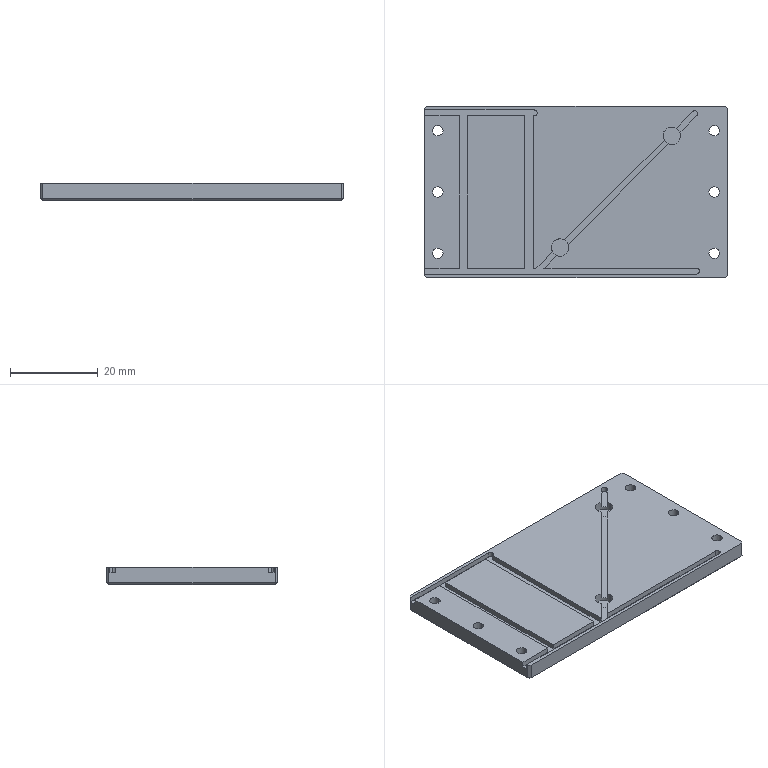Part | STEP file | ASND-0110-OPT-CO40-X-V1.0.5 side plate | 1 solid | 78 faces | box 69 x 39 x 4 mm | volume 10181 mm3 | plane 44 | cylinder 22 | cone 12 | commonest cylinder face diameters 2.4 x12 1.3 x6 4 x4